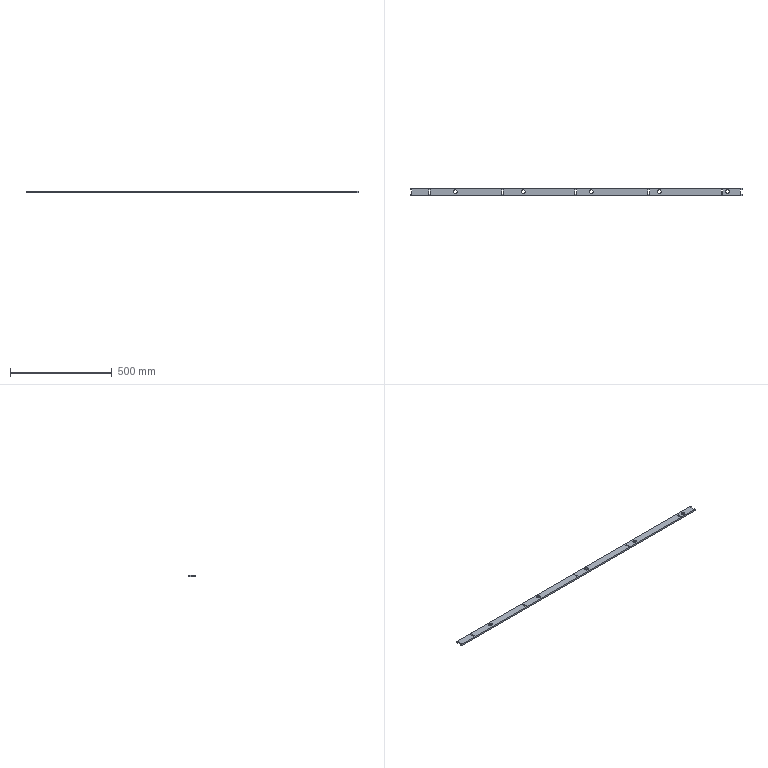Part | SolidWorks | features FlatPattern 1, SMBaseFlange 1, SheetMetal 1 | 1 solid | 44 faces | box 1635 x 34.8 x 8 mm | volume 435932 mm3 | plane 34 | cylinder 10 | commonest cylinder face diameters 18.1 x10
STEP:
#1=CARTESIAN_POINT('',(-81.05,53.917,8.));
#2=VERTEX_POINT('',#1);
#3=CARTESIAN_POINT('',(-62.95,53.917,8.));
#4=VERTEX_POINT('',#3);
#5=CARTESIAN_POINT('',(-72.,53.917,8.));
#6=DIRECTION('',(0.,0.,1.));
#7=DIRECTION('',(1.,0.,0.));
#8=AXIS2_PLACEMENT_3D('',#5,#6,#7);
#9=CIRCLE('',#8,9.05);
#10=EDGE_CURVE('',#2,#4,#9,.T.);
#11=ORIENTED_EDGE('',*,*,#10,.T.);
#12=CARTESIAN_POINT('',(-62.95,53.917,0.));
#13=VERTEX_POINT('',#12);
#14=CARTESIAN_POINT('',(-62.95,53.917,8.));
#15=DIRECTION('',(0.,0.,-1.));
#16=VECTOR('',#15,1000.);
#17=LINE('',#14,#16);
#18=EDGE_CURVE('',#4,#13,#17,.T.);
#19=ORIENTED_EDGE('',*,*,#18,.T.);
#20=CARTESIAN_POINT('',(-81.05,53.917,0.));
#21=VERTEX_POINT('',#20);
#22=CARTESIAN_POINT('',(-72.,53.917,0.));
#23=DIRECTION('',(0.,0.,1.));
#24=DIRECTION('',(1.,0.,0.));
#25=AXIS2_PLACEMENT_3D('',#22,#23,#24);
#26=CIRCLE('',#25,9.05);
#27=EDGE_CURVE('',#21,#13,#26,.T.);
#28=ORIENTED_EDGE('',*,*,#27,.F.);
#29=CARTESIAN_POINT('',(-81.05,53.917,8.));
#30=DIRECTION('',(0.,0.,-1.));
#31=VECTOR('',#30,1000.);
#32=LINE('',#29,#31);
#33=EDGE_CURVE('',#2,#21,#32,.T.);
#34=ORIENTED_EDGE('',*,*,#33,.F.);
#35=EDGE_LOOP('',(#11,#19,#28,#34));
#36=FACE_OUTER_BOUND('',#35,.T.);
#37=CARTESIAN_POINT('',(-72.,53.917,8.));
#38=DIRECTION('',(0.,0.,-1.));
#39=DIRECTION('',(-1.,0.,0.));
#40=AXIS2_PLACEMENT_3D('',#37,#38,#39);
#41=CYLINDRICAL_SURFACE('',#40,9.05);
#42=ADVANCED_FACE('',(#36),#41,.F.);
#43=CARTESIAN_POINT('',(-416.05,53.917,8.));
#44=VERTEX_POINT('',#43);
#45=CARTESIAN_POINT('',(-397.95,53.917,8.));
#46=VERTEX_POINT('',#45);
#47=CARTESIAN_POINT('',(-407.,53.917,8.));
#48=DIRECTION('',(0.,0.,1.));
#49=DIRECTION('',(1.,0.,0.));
#50=AXIS2_PLACEMENT_3D('',#47,#48,#49);
#51=CIRCLE('',#50,9.05);
#52=EDGE_CURVE('',#44,#46,#51,.T.);
#53=ORIENTED_EDGE('',*,*,#52,.T.);
#54=CARTESIAN_POINT('',(-397.95,53.917,0.));
#55=VERTEX_POINT('',#54);
#56=CARTESIAN_POINT('',(-397.95,53.917,8.));
#57=DIRECTION('',(0.,0.,-1.));
#58=VECTOR('',#57,1000.);
#59=LINE('',#56,#58);
#60=EDGE_CURVE('',#46,#55,#59,.T.);
#61=ORIENTED_EDGE('',*,*,#60,.T.);
#62=CARTESIAN_POINT('',(-416.05,53.917,0.));
#63=VERTEX_POINT('',#62);
#64=CARTESIAN_POINT('',(-407.,53.917,0.));
#65=DIRECTION('',(0.,0.,1.));
#66=DIRECTION('',(1.,0.,0.));
#67=AXIS2_PLACEMENT_3D('',#64,#65,#66);
#68=CIRCLE('',#67,9.05);
#69=EDGE_CURVE('',#63,#55,#68,.T.);
#70=ORIENTED_EDGE('',*,*,#69,.F.);
#71=CARTESIAN_POINT('',(-416.05,53.917,8.));
#72=DIRECTION('',(0.,0.,-1.));
#73=VECTOR('',#72,1000.);
#74=LINE('',#71,#73);
#75=EDGE_CURVE('',#44,#63,#74,.T.);
#76=ORIENTED_EDGE('',*,*,#75,.F.);
#77=EDGE_LOOP('',(#53,#61,#70,#76));
#78=FACE_OUTER_BOUND('',#77,.T.);
#79=CARTESIAN_POINT('',(-407.,53.917,8.));
#80=DIRECTION('',(0.,0.,-1.));
#81=DIRECTION('',(-1.,0.,0.));
#82=AXIS2_PLACEMENT_3D('',#79,#80,#81);
#83=CYLINDRICAL_SURFACE('',#82,9.05);
#84=ADVANCED_FACE('',(#78),#83,.F.);
#85=CARTESIAN_POINT('',(-751.05,53.917,8.));
#86=VERTEX_POINT('',#85);
#87=CARTESIAN_POINT('',(-732.95,53.917,8.));
#88=VERTEX_POINT('',#87);
#89=CARTESIAN_POINT('',(-742.,53.917,8.));
#90=DIRECTION('',(0.,0.,1.));
#91=DIRECTION('',(1.,0.,0.));
#92=AXIS2_PLACEMENT_3D('',#89,#90,#91);
#93=CIRCLE('',#92,9.05);
#94=EDGE_CURVE('',#86,#88,#93,.T.);
#95=ORIENTED_EDGE('',*,*,#94,.T.);
#96=CARTESIAN_POINT('',(-732.95,53.917,0.));
#97=VERTEX_POINT('',#96);
#98=CARTESIAN_POINT('',(-732.95,53.917,8.));
#99=DIRECTION('',(0.,0.,-1.));
#100=VECTOR('',#99,1000.);
#101=LINE('',#98,#100);
#102=EDGE_CURVE('',#88,#97,#101,.T.);
#103=ORIENTED_EDGE('',*,*,#102,.T.);
#104=CARTESIAN_POINT('',(-751.05,53.917,0.));
#105=VERTEX_POINT('',#104);
#106=CARTESIAN_POINT('',(-742.,53.917,0.));
#107=DIRECTION('',(0.,0.,1.));
#108=DIRECTION('',(1.,0.,0.));
#109=AXIS2_PLACEMENT_3D('',#106,#107,#108);
#110=CIRCLE('',#109,9.05);
#111=EDGE_CURVE('',#105,#97,#110,.T.);
#112=ORIENTED_EDGE('',*,*,#111,.F.);
#113=CARTESIAN_POINT('',(-751.05,53.917,8.));
#114=DIRECTION('',(0.,0.,-1.));
#115=VECTOR('',#114,1000.);
#116=LINE('',#113,#115);
#117=EDGE_CURVE('',#86,#105,#116,.T.);
#118=ORIENTED_EDGE('',*,*,#117,.F.);
#119=EDGE_LOOP('',(#95,#103,#112,#118));
#120=FACE_OUTER_BOUND('',#119,.T.);
#121=CARTESIAN_POINT('',(-742.,53.917,8.));
#122=DIRECTION('',(0.,0.,-1.));
#123=DIRECTION('',(-1.,0.,0.));
#124=AXIS2_PLACEMENT_3D('',#121,#122,#123);
#125=CYLINDRICAL_SURFACE('',#124,9.05);
#126=ADVANCED_FACE('',(#120),#125,.F.);
#127=CARTESIAN_POINT('',(-1086.05,53.917,8.));
#128=VERTEX_POINT('',#127);
#129=CARTESIAN_POINT('',(-1067.95,53.917,8.));
#130=VERTEX_POINT('',#129);
#131=CARTESIAN_POINT('',(-1077.,53.917,8.));
#132=DIRECTION('',(0.,0.,1.));
#133=DIRECTION('',(1.,0.,0.));
#134=AXIS2_PLACEMENT_3D('',#131,#132,#133);
#135=CIRCLE('',#134,9.05);
#136=EDGE_CURVE('',#128,#130,#135,.T.);
#137=ORIENTED_EDGE('',*,*,#136,.T.);
#138=CARTESIAN_POINT('',(-1067.95,53.917,0.));
#139=VERTEX_POINT('',#138);
#140=CARTESIAN_POINT('',(-1067.95,53.917,8.));
#141=DIRECTION('',(0.,0.,-1.));
#142=VECTOR('',#141,1000.);
#143=LINE('',#140,#142);
#144=EDGE_CURVE('',#130,#139,#143,.T.);
#145=ORIENTED_EDGE('',*,*,#144,.T.);
#146=CARTESIAN_POINT('',(-1086.05,53.917,0.));
#147=VERTEX_POINT('',#146);
#148=CARTESIAN_POINT('',(-1077.,53.917,0.));
#149=DIRECTION('',(0.,0.,1.));
#150=DIRECTION('',(1.,0.,0.));
#151=AXIS2_PLACEMENT_3D('',#148,#149,#150);
#152=CIRCLE('',#151,9.05);
#153=EDGE_CURVE('',#147,#139,#152,.T.);
#154=ORIENTED_EDGE('',*,*,#153,.F.);
#155=CARTESIAN_POINT('',(-1086.05,53.917,8.));
#156=DIRECTION('',(0.,0.,-1.));
#157=VECTOR('',#156,1000.);
#158=LINE('',#155,#157);
#159=EDGE_CURVE('',#128,#147,#158,.T.);
#160=ORIENTED_EDGE('',*,*,#159,.F.);
#161=EDGE_LOOP('',(#137,#145,#154,#160));
#162=FACE_OUTER_BOUND('',#161,.T.);
#163=CARTESIAN_POINT('',(-1077.,53.917,8.));
#164=DIRECTION('',(0.,0.,-1.));
#165=DIRECTION('',(-1.,0.,0.));
#166=AXIS2_PLACEMENT_3D('',#163,#164,#165);
#167=CYLINDRICAL_SURFACE('',#166,9.05);
#168=ADVANCED_FACE('',(#162),#167,.F.);
#169=CARTESIAN_POINT('',(-1421.05,53.917,8.));
#170=VERTEX_POINT('',#169);
#171=CARTESIAN_POINT('',(-1402.95,53.917,8.));
#172=VERTEX_POINT('',#171);
#173=CARTESIAN_POINT('',(-1412.,53.917,8.));
#174=DIRECTION('',(0.,0.,1.));
#175=DIRECTION('',(1.,0.,0.));
#176=AXIS2_PLACEMENT_3D('',#173,#174,#175);
#177=CIRCLE('',#176,9.05);
#178=EDGE_CURVE('',#170,#172,#177,.T.);
#179=ORIENTED_EDGE('',*,*,#178,.T.);
#180=CARTESIAN_POINT('',(-1402.95,53.917,0.));
#181=VERTEX_POINT('',#180);
#182=CARTESIAN_POINT('',(-1402.95,53.917,8.));
#183=DIRECTION('',(0.,0.,-1.));
#184=VECTOR('',#183,1000.);
#185=LINE('',#182,#184);
#186=EDGE_CURVE('',#172,#181,#185,.T.);
#187=ORIENTED_EDGE('',*,*,#186,.T.);
#188=CARTESIAN_POINT('',(-1421.05,53.917,0.));
#189=VERTEX_POINT('',#188);
#190=CARTESIAN_POINT('',(-1412.,53.917,0.));
#191=DIRECTION('',(0.,0.,1.));
#192=DIRECTION('',(1.,0.,0.));
#193=AXIS2_PLACEMENT_3D('',#190,#191,#192);
#194=CIRCLE('',#193,9.05);
#195=EDGE_CURVE('',#189,#181,#194,.T.);
#196=ORIENTED_EDGE('',*,*,#195,.F.);
#197=CARTESIAN_POINT('',(-1421.05,53.917,8.));
#198=DIRECTION('',(0.,0.,-1.));
#199=VECTOR('',#198,1000.);
#200=LINE('',#197,#199);
#201=EDGE_CURVE('',#170,#189,#200,.T.);
#202=ORIENTED_EDGE('',*,*,#201,.F.);
#203=EDGE_LOOP('',(#179,#187,#196,#202));
#204=FACE_OUTER_BOUND('',#203,.T.);
#205=CARTESIAN_POINT('',(-1412.,53.917,8.));
#206=DIRECTION('',(0.,0.,-1.));
#207=DIRECTION('',(-1.,0.,0.));
#208=AXIS2_PLACEMENT_3D('',#205,#206,#207);
#209=CYLINDRICAL_SURFACE('',#208,9.05);
#210=ADVANCED_FACE('',(#204),#209,.F.);
#211=ORIENTED_EDGE('',*,*,#52,.F.);
#212=CARTESIAN_POINT('',(-407.,53.917,8.));
#213=DIRECTION('',(0.,0.,1.));
#214=DIRECTION('',(1.,0.,0.));
#215=AXIS2_PLACEMENT_3D('',#212,#213,#214);
#216=CIRCLE('',#215,9.05);
#217=EDGE_CURVE('',#46,#44,#216,.T.);
#218=ORIENTED_EDGE('',*,*,#217,.F.);
#219=EDGE_LOOP('',(#211,#218));
#220=FACE_BOUND('',#219,.T.);
#221=ORIENTED_EDGE('',*,*,#136,.F.);
#222=CARTESIAN_POINT('',(-1077.,53.917,8.));
#223=DIRECTION('',(0.,0.,1.));
#224=DIRECTION('',(1.,0.,0.));
#225=AXIS2_PLACEMENT_3D('',#222,#223,#224);
#226=CIRCLE('',#225,9.05);
#227=EDGE_CURVE('',#130,#128,#226,.T.);
#228=ORIENTED_EDGE('',*,*,#227,.F.);
#229=EDGE_LOOP('',(#221,#228));
#230=FACE_BOUND('',#229,.T.);
#231=CARTESIAN_POINT('',(0.,62.417,8.));
#232=VERTEX_POINT('',#231);
#233=CARTESIAN_POINT('',(0.,69.917,8.));
#234=VERTEX_POINT('',#233);
#235=CARTESIAN_POINT('',(0.,69.917,8.));
#236=DIRECTION('',(0.,1.,0.));
#237=VECTOR('',#236,1000.);
#238=LINE('',#235,#237);
#239=EDGE_CURVE('',#232,#234,#238,.T.);
#240=ORIENTED_EDGE('',*,*,#239,.T.);
#241=CARTESIAN_POINT('',(-1635.,69.917,8.));
#242=VERTEX_POINT('',#241);
#243=CARTESIAN_POINT('',(0.,69.917,8.));
#244=DIRECTION('',(-1.,0.,0.));
#245=VECTOR('',#244,1000.);
#246=LINE('',#243,#245);
#247=EDGE_CURVE('',#234,#242,#246,.T.);
#248=ORIENTED_EDGE('',*,*,#247,.T.);
#249=CARTESIAN_POINT('',(-1635.,62.417,8.));
#250=VERTEX_POINT('',#249);
#251=CARTESIAN_POINT('',(-1635.,69.917,8.));
#252=DIRECTION('',(0.,-1.,0.));
#253=VECTOR('',#252,1000.);
#254=LINE('',#251,#253);
#255=EDGE_CURVE('',#242,#250,#254,.T.);
#256=ORIENTED_EDGE('',*,*,#255,.T.);
#257=CARTESIAN_POINT('',(-1627.,62.417,8.));
#258=VERTEX_POINT('',#257);
#259=CARTESIAN_POINT('',(-1627.,62.417,8.));
#260=DIRECTION('',(1.,0.,0.));
#261=VECTOR('',#260,1000.);
#262=LINE('',#259,#261);
#263=EDGE_CURVE('',#250,#258,#262,.T.);
#264=ORIENTED_EDGE('',*,*,#263,.T.);
#265=CARTESIAN_POINT('',(-1627.,42.417,8.));
#266=VERTEX_POINT('',#265);
#267=CARTESIAN_POINT('',(-1627.,62.417,8.));
#268=DIRECTION('',(0.,-1.,0.));
#269=VECTOR('',#268,1000.);
#270=LINE('',#267,#269);
#271=EDGE_CURVE('',#258,#266,#270,.T.);
#272=ORIENTED_EDGE('',*,*,#271,.T.);
#273=CARTESIAN_POINT('',(-1635.,42.417,8.));
#274=VERTEX_POINT('',#273);
#275=CARTESIAN_POINT('',(-1627.,42.417,8.));
#276=DIRECTION('',(-1.,0.,0.));
#277=VECTOR('',#276,1000.);
#278=LINE('',#275,#277);
#279=EDGE_CURVE('',#266,#274,#278,.T.);
#280=ORIENTED_EDGE('',*,*,#279,.T.);
#281=CARTESIAN_POINT('',(-1635.,35.117,8.));
#282=VERTEX_POINT('',#281);
#283=CARTESIAN_POINT('',(-1635.,42.417,8.));
#284=DIRECTION('',(0.,-1.,0.));
#285=VECTOR('',#284,1000.);
#286=LINE('',#283,#285);
#287=EDGE_CURVE('',#274,#282,#286,.T.);
#288=ORIENTED_EDGE('',*,*,#287,.T.);
#289=CARTESIAN_POINT('',(0.,35.117,8.));
#290=VERTEX_POINT('',#289);
#291=CARTESIAN_POINT('',(0.,35.117,8.));
#292=DIRECTION('',(1.,0.,0.));
#293=VECTOR('',#292,1000.);
#294=LINE('',#291,#293);
#295=EDGE_CURVE('',#282,#290,#294,.T.);
#296=ORIENTED_EDGE('',*,*,#295,.T.);
#297=CARTESIAN_POINT('',(0.,42.417,8.));
#298=VERTEX_POINT('',#297);
#299=CARTESIAN_POINT('',(0.,42.417,8.));
#300=DIRECTION('',(0.,1.,0.));
#301=VECTOR('',#300,1000.);
#302=LINE('',#299,#301);
#303=EDGE_CURVE('',#290,#298,#302,.T.);
#304=ORIENTED_EDGE('',*,*,#303,.T.);
#305=CARTESIAN_POINT('',(-8.,42.417,8.));
#306=VERTEX_POINT('',#305);
#307=CARTESIAN_POINT('',(-8.,42.417,8.));
#308=DIRECTION('',(-1.,0.,0.));
#309=VECTOR('',#308,1000.);
#310=LINE('',#307,#309);
#311=EDGE_CURVE('',#298,#306,#310,.T.);
#312=ORIENTED_EDGE('',*,*,#311,.T.);
#313=CARTESIAN_POINT('',(-8.,62.417,8.));
#314=VERTEX_POINT('',#313);
#315=CARTESIAN_POINT('',(-8.,62.417,8.));
#316=DIRECTION('',(0.,1.,0.));
#317=VECTOR('',#316,1000.);
#318=LINE('',#315,#317);
#319=EDGE_CURVE('',#306,#314,#318,.T.);
#320=ORIENTED_EDGE('',*,*,#319,.T.);
#321=CARTESIAN_POINT('',(-8.,62.417,8.));
#322=DIRECTION('',(1.,0.,0.));
#323=VECTOR('',#322,1000.);
#324=LINE('',#321,#323);
#325=EDGE_CURVE('',#314,#232,#324,.T.);
#326=ORIENTED_EDGE('',*,*,#325,.T.);
#327=EDGE_LOOP('',(#240,#248,#256,#264,#272,#280,#288,#296,#304,#312,#320,#326));
#328=FACE_OUTER_BOUND('',#327,.T.);
#329=ORIENTED_EDGE('',*,*,#178,.F.);
#330=CARTESIAN_POINT('',(-1412.,53.917,8.));
#331=DIRECTION('',(0.,0.,1.));
#332=DIRECTION('',(1.,0.,0.));
#333=AXIS2_PLACEMENT_3D('',#330,#331,#332);
#334=CIRCLE('',#333,9.05);
#335=EDGE_CURVE('',#172,#170,#334,.T.);
#336=ORIENTED_EDGE('',*,*,#335,.F.);
#337=EDGE_LOOP('',(#329,#336));
#338=FACE_BOUND('',#337,.T.);
#339=ORIENTED_EDGE('',*,*,#94,.F.);
#340=CARTESIAN_POINT('',(-742.,53.917,8.));
#341=DIRECTION('',(0.,0.,1.));
#342=DIRECTION('',(1.,0.,0.));
#343=AXIS2_PLACEMENT_3D('',#340,#341,#342);
#344=CIRCLE('',#343,9.05);
#345=EDGE_CURVE('',#88,#86,#344,.T.);
#346=ORIENTED_EDGE('',*,*,#345,.F.);
#347=EDGE_LOOP('',(#339,#346));
#348=FACE_BOUND('',#347,.T.);
#349=ORIENTED_EDGE('',*,*,#10,.F.);
#350=CARTESIAN_POINT('',(-72.,53.917,8.));
#351=DIRECTION('',(0.,0.,1.));
#352=DIRECTION('',(1.,0.,0.));
#353=AXIS2_PLACEMENT_3D('',#350,#351,#352);
#354=CIRCLE('',#353,9.05);
#355=EDGE_CURVE('',#4,#2,#354,.T.);
#356=ORIENTED_EDGE('',*,*,#355,.F.);
#357=EDGE_LOOP('',(#349,#356));
#358=FACE_BOUND('',#357,.T.);
#359=CARTESIAN_POINT('',(-95.,62.417,8.));
#360=VERTEX_POINT('',#359);
#361=CARTESIAN_POINT('',(-103.,62.417,8.));
#362=VERTEX_POINT('',#361);
#363=CARTESIAN_POINT('',(-95.,62.417,8.));
#364=DIRECTION('',(-1.,0.,0.));
#365=VECTOR('',#364,1000.);
#366=LINE('',#363,#365);
#367=EDGE_CURVE('',#360,#362,#366,.T.);
#368=ORIENTED_EDGE('',*,*,#367,.F.);
#369=CARTESIAN_POINT('',(-95.,42.417,8.));
#370=VERTEX_POINT('',#369);
#371=CARTESIAN_POINT('',(-95.,62.417,8.));
#372=DIRECTION('',(0.,1.,0.));
#373=VECTOR('',#372,1000.);
#374=LINE('',#371,#373);
#375=EDGE_CURVE('',#370,#360,#374,.T.);
#376=ORIENTED_EDGE('',*,*,#375,.F.);
#377=CARTESIAN_POINT('',(-103.,42.417,8.));
#378=VERTEX_POINT('',#377);
#379=CARTESIAN_POINT('',(-95.,42.417,8.));
#380=DIRECTION('',(1.,0.,0.));
#381=VECTOR('',#380,1000.);
#382=LINE('',#379,#381);
#383=EDGE_CURVE('',#378,#370,#382,.T.);
#384=ORIENTED_EDGE('',*,*,#383,.F.);
#385=CARTESIAN_POINT('',(-103.,62.417,8.));
#386=DIRECTION('',(0.,-1.,0.));
#387=VECTOR('',#386,1000.);
#388=LINE('',#385,#387);
#389=EDGE_CURVE('',#362,#378,#388,.T.);
#390=ORIENTED_EDGE('',*,*,#389,.F.);
#391=EDGE_LOOP('',(#368,#376,#384,#390));
#392=FACE_BOUND('',#391,.T.);
#393=CARTESIAN_POINT('',(-455.,62.417,8.));
#394=VERTEX_POINT('',#393);
#395=CARTESIAN_POINT('',(-463.,62.417,8.));
#396=VERTEX_POINT('',#395);
#397=CARTESIAN_POINT('',(-455.,62.417,8.));
#398=DIRECTION('',(-1.,0.,0.));
#399=VECTOR('',#398,1000.);
#400=LINE('',#397,#399);
#401=EDGE_CURVE('',#394,#396,#400,.T.);
#402=ORIENTED_EDGE('',*,*,#401,.F.);
#403=CARTESIAN_POINT('',(-455.,42.417,8.));
#404=VERTEX_POINT('',#403);
#405=CARTESIAN_POINT('',(-455.,62.417,8.));
#406=DIRECTION('',(0.,1.,0.));
#407=VECTOR('',#406,1000.);
#408=LINE('',#405,#407);
#409=EDGE_CURVE('',#404,#394,#408,.T.);
#410=ORIENTED_EDGE('',*,*,#409,.F.);
#411=CARTESIAN_POINT('',(-463.,42.417,8.));
#412=VERTEX_POINT('',#411);
#413=CARTESIAN_POINT('',(-455.,42.417,8.));
#414=DIRECTION('',(1.,0.,0.));
#415=VECTOR('',#414,1000.);
#416=LINE('',#413,#415);
#417=EDGE_CURVE('',#412,#404,#416,.T.);
#418=ORIENTED_EDGE('',*,*,#417,.F.);
#419=CARTESIAN_POINT('',(-463.,62.417,8.));
#420=DIRECTION('',(0.,-1.,0.));
#421=VECTOR('',#420,1000.);
#422=LINE('',#419,#421);
#423=EDGE_CURVE('',#396,#412,#422,.T.);
#424=ORIENTED_EDGE('',*,*,#423,.F.);
#425=EDGE_LOOP('',(#402,#410,#418,#424));
#426=FACE_BOUND('',#425,.T.);
#427=CARTESIAN_POINT('',(-815.,62.417,8.));
#428=VERTEX_POINT('',#427);
#429=CARTESIAN_POINT('',(-823.,62.417,8.));
#430=VERTEX_POINT('',#429);
#431=CARTESIAN_POINT('',(-815.,62.417,8.));
#432=DIRECTION('',(-1.,0.,0.));
#433=VECTOR('',#432,1000.);
#434=LINE('',#431,#433);
#435=EDGE_CURVE('',#428,#430,#434,.T.);
#436=ORIENTED_EDGE('',*,*,#435,.F.);
#437=CARTESIAN_POINT('',(-815.,42.417,8.));
#438=VERTEX_POINT('',#437);
#439=CARTESIAN_POINT('',(-815.,62.417,8.));
#440=DIRECTION('',(0.,1.,0.));
#441=VECTOR('',#440,1000.);
#442=LINE('',#439,#441);
#443=EDGE_CURVE('',#438,#428,#442,.T.);
#444=ORIENTED_EDGE('',*,*,#443,.F.);
#445=CARTESIAN_POINT('',(-823.,42.417,8.));
#446=VERTEX_POINT('',#445);
#447=CARTESIAN_POINT('',(-815.,42.417,8.));
#448=DIRECTION('',(1.,0.,0.));
#449=VECTOR('',#448,1000.);
#450=LINE('',#447,#449);
#451=EDGE_CURVE('',#446,#438,#450,.T.);
#452=ORIENTED_EDGE('',*,*,#451,.F.);
#453=CARTESIAN_POINT('',(-823.,62.417,8.));
#454=DIRECTION('',(0.,-1.,0.));
#455=VECTOR('',#454,1000.);
#456=LINE('',#453,#455);
#457=EDGE_CURVE('',#430,#446,#456,.T.);
#458=ORIENTED_EDGE('',*,*,#457,.F.);
#459=EDGE_LOOP('',(#436,#444,#452,#458));
#460=FACE_BOUND('',#459,.T.);
#461=CARTESIAN_POINT('',(-1175.,62.417,8.));
#462=VERTEX_POINT('',#461);
#463=CARTESIAN_POINT('',(-1183.,62.417,8.));
#464=VERTEX_POINT('',#463);
#465=CARTESIAN_POINT('',(-1175.,62.417,8.));
#466=DIRECTION('',(-1.,0.,0.));
#467=VECTOR('',#466,1000.);
#468=LINE('',#465,#467);
#469=EDGE_CURVE('',#462,#464,#468,.T.);
#470=ORIENTED_EDGE('',*,*,#469,.F.);
#471=CARTESIAN_POINT('',(-1175.,42.417,8.));
#472=VERTEX_POINT('',#471);
#473=CARTESIAN_POINT('',(-1175.,62.417,8.));
#474=DIRECTION('',(0.,1.,0.));
#475=VECTOR('',#474,1000.);
#476=LINE('',#473,#475);
#477=EDGE_CURVE('',#472,#462,#476,.T.);
#478=ORIENTED_EDGE('',*,*,#477,.F.);
#479=CARTESIAN_POINT('',(-1183.,42.417,8.));
#480=VERTEX_POINT('',#479);
#481=CARTESIAN_POINT('',(-1175.,42.417,8.));
#482=DIRECTION('',(1.,0.,0.));
#483=VECTOR('',#482,1000.);
#484=LINE('',#481,#483);
#485=EDGE_CURVE('',#480,#472,#484,.T.);
#486=ORIENTED_EDGE('',*,*,#485,.F.);
#487=CARTESIAN_POINT('',(-1183.,62.417,8.));
#488=DIRECTION('',(0.,-1.,0.));
#489=VECTOR('',#488,1000.);
#490=LINE('',#487,#489);
#491=EDGE_CURVE('',#464,#480,#490,.T.);
#492=ORIENTED_EDGE('',*,*,#491,.F.);
#493=EDGE_LOOP('',(#470,#478,#486,#492));
#494=FACE_BOUND('',#493,.T.);
#495=CARTESIAN_POINT('',(-1535.,62.417,8.));
#496=VERTEX_POINT('',#495);
#497=CARTESIAN_POINT('',(-1543.,62.417,8.));
#498=VERTEX_POINT('',#497);
#499=CARTESIAN_POINT('',(-1535.,62.417,8.));
#500=DIRECTION('',(-1.,0.,0.));
#501=VECTOR('',#500,1000.);
#502=LINE('',#499,#501);
#503=EDGE_CURVE('',#496,#498,#502,.T.);
#504=ORIENTED_EDGE('',*,*,#503,.F.);
#505=CARTESIAN_POINT('',(-1535.,42.417,8.));
#506=VERTEX_POINT('',#505);
#507=CARTESIAN_POINT('',(-1535.,62.417,8.));
#508=DIRECTION('',(0.,1.,0.));
#509=VECTOR('',#508,1000.);
#510=LINE('',#507,#509);
#511=EDGE_CURVE('',#506,#496,#510,.T.);
#512=ORIENTED_EDGE('',*,*,#511,.F.);
#513=CARTESIAN_POINT('',(-1543.,42.417,8.));
#514=VERTEX_POINT('',#513);
#515=CARTESIAN_POINT('',(-1535.,42.417,8.));
#516=DIRECTION('',(1.,0.,0.));
#517=VECTOR('',#516,1000.);
#518=LINE('',#515,#517);
#519=EDGE_CURVE('',#514,#506,#518,.T.);
#520=ORIENTED_EDGE('',*,*,#519,.F.);
#521=CARTESIAN_POINT('',(-1543.,62.417,8.));
#522=DIRECTION('',(0.,-1.,0.));
#523=VECTOR('',#522,1000.);
#524=LINE('',#521,#523);
#525=EDGE_CURVE('',#498,#514,#524,.T.);
#526=ORIENTED_EDGE('',*,*,#525,.F.);
#527=EDGE_LOOP('',(#504,#512,#520,#526));
#528=FACE_BOUND('',#527,.T.);
#529=CARTESIAN_POINT('',(0.,0.,8.));
#530=DIRECTION('',(0.,0.,1.));
#531=DIRECTION('',(1.,0.,0.));
#532=AXIS2_PLACEMENT_3D('',#529,#530,#531);
#533=PLANE('',#532);
#534=ADVANCED_FACE('',(#220,#230,#328,#338,#348,#358,#392,#426,#460,#494,#528),#533,.T.);
#535=CARTESIAN_POINT('',(-1175.,42.417,0.));
#536=VERTEX_POINT('',#535);
#537=CARTESIAN_POINT('',(-1175.,62.417,0.));
#538=VERTEX_POINT('',#537);
#539=CARTESIAN_POINT('',(-1175.,62.417,0.));
#540=DIRECTION('',(0.,1.,0.));
#541=VECTOR('',#540,1000.);
#542=LINE('',#539,#541);
#543=EDGE_CURVE('',#536,#538,#542,.T.);
#544=ORIENTED_EDGE('',*,*,#543,.T.);
#545=CARTESIAN_POINT('',(-1183.,62.417,0.));
#546=VERTEX_POINT('',#545);
#547=CARTESIAN_POINT('',(-1175.,62.417,0.));
#548=DIRECTION('',(-1.,0.,0.));
#549=VECTOR('',#548,1000.);
#550=LINE('',#547,#549);
#551=EDGE_CURVE('',#538,#546,#550,.T.);
#552=ORIENTED_EDGE('',*,*,#551,.T.);
#553=CARTESIAN_POINT('',(-1183.,42.417,0.));
#554=VERTEX_POINT('',#553);
#555=CARTESIAN_POINT('',(-1183.,62.417,0.));
#556=DIRECTION('',(0.,-1.,0.));
#557=VECTOR('',#556,1000.);
#558=LINE('',#555,#557);
#559=EDGE_CURVE('',#546,#554,#558,.T.);
#560=ORIENTED_EDGE('',*,*,#559,.T.);
#561=CARTESIAN_POINT('',(-1175.,42.417,0.));
#562=DIRECTION('',(1.,0.,0.));
#563=VECTOR('',#562,1000.);
#564=LINE('',#561,#563);
#565=EDGE_CURVE('',#554,#536,#564,.T.);
#566=ORIENTED_EDGE('',*,*,#565,.T.);
#567=EDGE_LOOP('',(#544,#552,#560,#566));
#568=FACE_BOUND('',#567,.T.);
#569=CARTESIAN_POINT('',(-455.,42.417,0.));
#570=VERTEX_POINT('',#569);
#571=CARTESIAN_POINT('',(-455.,62.417,0.));
#572=VERTEX_POINT('',#571);
#573=CARTESIAN_POINT('',(-455.,62.417,0.));
#574=DIRECTION('',(0.,1.,0.));
#575=VECTOR('',#574,1000.);
#576=LINE('',#573,#575);
#577=EDGE_CURVE('',#570,#572,#576,.T.);
#578=ORIENTED_EDGE('',*,*,#577,.T.);
#579=CARTESIAN_POINT('',(-463.,62.417,0.));
#580=VERTEX_POINT('',#579);
#581=CARTESIAN_POINT('',(-455.,62.417,0.));
#582=DIRECTION('',(-1.,0.,0.));
#583=VECTOR('',#582,1000.);
#584=LINE('',#581,#583);
#585=EDGE_CURVE('',#572,#580,#584,.T.);
#586=ORIENTED_EDGE('',*,*,#585,.T.);
#587=CARTESIAN_POINT('',(-463.,42.417,0.));
#588=VERTEX_POINT('',#587);
#589=CARTESIAN_POINT('',(-463.,62.417,0.));
#590=DIRECTION('',(0.,-1.,0.));
#591=VECTOR('',#590,1000.);
#592=LINE('',#589,#591);
#593=EDGE_CURVE('',#580,#588,#592,.T.);
#594=ORIENTED_EDGE('',*,*,#593,.T.);
#595=CARTESIAN_POINT('',(-455.,42.417,0.));
#596=DIRECTION('',(1.,0.,0.));
#597=VECTOR('',#596,1000.);
#598=LINE('',#595,#597);
#599=EDGE_CURVE('',#588,#570,#598,.T.);
#600=ORIENTED_EDGE('',*,*,#599,.T.);
#601=EDGE_LOOP('',(#578,#586,#594,#600));
#602=FACE_BOUND('',#601,.T.);
#603=ORIENTED_EDGE('',*,*,#27,.T.);
#604=CARTESIAN_POINT('',(-72.,53.917,0.));
#605=DIRECTION('',(0.,0.,1.));
#606=DIRECTION('',(1.,0.,0.));
#607=AXIS2_PLACEMENT_3D('',#604,#605,#606);
#608=CIRCLE('',#607,9.05);
#609=EDGE_CURVE('',#13,#21,#608,.T.);
#610=ORIENTED_EDGE('',*,*,#609,.T.);
#611=EDGE_LOOP('',(#603,#610));
#612=FACE_BOUND('',#611,.T.);
#613=ORIENTED_EDGE('',*,*,#69,.T.);
#614=CARTESIAN_POINT('',(-407.,53.917,0.));
#615=DIRECTION('',(0.,0.,1.));
#616=DIRECTION('',(1.,0.,0.));
#617=AXIS2_PLACEMENT_3D('',#614,#615,#616);
#618=CIRCLE('',#617,9.05);
#619=EDGE_CURVE('',#55,#63,#618,.T.);
#620=ORIENTED_EDGE('',*,*,#619,.T.);
#621=EDGE_LOOP('',(#613,#620));
#622=FACE_BOUND('',#621,.T.);
#623=ORIENTED_EDGE('',*,*,#111,.T.);
#624=CARTESIAN_POINT('',(-742.,53.917,0.));
#625=DIRECTION('',(0.,0.,1.));
#626=DIRECTION('',(1.,0.,0.));
#627=AXIS2_PLACEMENT_3D('',#624,#625,#626);
#628=CIRCLE('',#627,9.05);
#629=EDGE_CURVE('',#97,#105,#628,.T.);
#630=ORIENTED_EDGE('',*,*,#629,.T.);
#631=EDGE_LOOP('',(#623,#630));
#632=FACE_BOUND('',#631,.T.);
#633=ORIENTED_EDGE('',*,*,#153,.T.);
#634=CARTESIAN_POINT('',(-1077.,53.917,0.));
#635=DIRECTION('',(0.,0.,1.));
#636=DIRECTION('',(1.,0.,0.));
#637=AXIS2_PLACEMENT_3D('',#634,#635,#636);
#638=CIRCLE('',#637,9.05);
#639=EDGE_CURVE('',#139,#147,#638,.T.);
#640=ORIENTED_EDGE('',*,*,#639,.T.);
#641=EDGE_LOOP('',(#633,#640));
#642=FACE_BOUND('',#641,.T.);
#643=ORIENTED_EDGE('',*,*,#195,.T.);
#644=CARTESIAN_POINT('',(-1412.,53.917,0.));
#645=DIRECTION('',(0.,0.,1.));
#646=DIRECTION('',(1.,0.,0.));
#647=AXIS2_PLACEMENT_3D('',#644,#645,#646);
#648=CIRCLE('',#647,9.05);
#649=EDGE_CURVE('',#181,#189,#648,.T.);
#650=ORIENTED_EDGE('',*,*,#649,.T.);
#651=EDGE_LOOP('',(#643,#650));
#652=FACE_BOUND('',#651,.T.);
#653=CARTESIAN_POINT('',(0.,62.417,0.));
#654=VERTEX_POINT('',#653);
#655=CARTESIAN_POINT('',(0.,69.917,0.));
#656=VERTEX_POINT('',#655);
#657=CARTESIAN_POINT('',(0.,69.917,0.));
#658=DIRECTION('',(0.,1.,0.));
#659=VECTOR('',#658,1000.);
#660=LINE('',#657,#659);
#661=EDGE_CURVE('',#654,#656,#660,.T.);
#662=ORIENTED_EDGE('',*,*,#661,.F.);
#663=CARTESIAN_POINT('',(-8.,62.417,0.));
#664=VERTEX_POINT('',#663);
#665=CARTESIAN_POINT('',(-8.,62.417,0.));
#666=DIRECTION('',(1.,0.,0.));
#667=VECTOR('',#666,1000.);
#668=LINE('',#665,#667);
#669=EDGE_CURVE('',#664,#654,#668,.T.);
#670=ORIENTED_EDGE('',*,*,#669,.F.);
#671=CARTESIAN_POINT('',(-8.,42.417,0.));
#672=VERTEX_POINT('',#671);
#673=CARTESIAN_POINT('',(-8.,62.417,0.));
#674=DIRECTION('',(0.,1.,0.));
#675=VECTOR('',#674,1000.);
#676=LINE('',#673,#675);
#677=EDGE_CURVE('',#672,#664,#676,.T.);
#678=ORIENTED_EDGE('',*,*,#677,.F.);
#679=CARTESIAN_POINT('',(0.,42.417,0.));
#680=VERTEX_POINT('',#679);
#681=CARTESIAN_POINT('',(-8.,42.417,0.));
#682=DIRECTION('',(-1.,0.,0.));
#683=VECTOR('',#682,1000.);
#684=LINE('',#681,#683);
#685=EDGE_CURVE('',#680,#672,#684,.T.);
#686=ORIENTED_EDGE('',*,*,#685,.F.);
#687=CARTESIAN_POINT('',(0.,35.117,0.));
#688=VERTEX_POINT('',#687);
#689=CARTESIAN_POINT('',(0.,42.417,0.));
#690=DIRECTION('',(0.,1.,0.));
#691=VECTOR('',#690,1000.);
#692=LINE('',#689,#691);
#693=EDGE_CURVE('',#688,#680,#692,.T.);
#694=ORIENTED_EDGE('',*,*,#693,.F.);
#695=CARTESIAN_POINT('',(-1635.,35.117,0.));
#696=VERTEX_POINT('',#695);
#697=CARTESIAN_POINT('',(0.,35.117,0.));
#698=DIRECTION('',(1.,0.,0.));
#699=VECTOR('',#698,1000.);
#700=LINE('',#697,#699);
#701=EDGE_CURVE('',#696,#688,#700,.T.);
#702=ORIENTED_EDGE('',*,*,#701,.F.);
#703=CARTESIAN_POINT('',(-1635.,42.417,0.));
#704=VERTEX_POINT('',#703);
#705=CARTESIAN_POINT('',(-1635.,42.417,0.));
#706=DIRECTION('',(0.,-1.,0.));
#707=VECTOR('',#706,1000.);
#708=LINE('',#705,#707);
#709=EDGE_CURVE('',#704,#696,#708,.T.);
#710=ORIENTED_EDGE('',*,*,#709,.F.);
#711=CARTESIAN_POINT('',(-1627.,42.417,0.));
#712=VERTEX_POINT('',#711);
#713=CARTESIAN_POINT('',(-1627.,42.417,0.));
#714=DIRECTION('',(-1.,0.,0.));
#715=VECTOR('',#714,1000.);
#716=LINE('',#713,#715);
#717=EDGE_CURVE('',#712,#704,#716,.T.);
#718=ORIENTED_EDGE('',*,*,#717,.F.);
#719=CARTESIAN_POINT('',(-1627.,62.417,0.));
#720=VERTEX_POINT('',#719);
#721=CARTESIAN_POINT('',(-1627.,62.417,0.));
#722=DIRECTION('',(0.,-1.,0.));
#723=VECTOR('',#722,1000.);
#724=LINE('',#721,#723);
#725=EDGE_CURVE('',#720,#712,#724,.T.);
#726=ORIENTED_EDGE('',*,*,#725,.F.);
#727=CARTESIAN_POINT('',(-1635.,62.417,0.));
#728=VERTEX_POINT('',#727);
#729=CARTESIAN_POINT('',(-1627.,62.417,0.));
#730=DIRECTION('',(1.,0.,0.));
#731=VECTOR('',#730,1000.);
#732=LINE('',#729,#731);
#733=EDGE_CURVE('',#728,#720,#732,.T.);
#734=ORIENTED_EDGE('',*,*,#733,.F.);
#735=CARTESIAN_POINT('',(-1635.,69.917,0.));
#736=VERTEX_POINT('',#735);
#737=CARTESIAN_POINT('',(-1635.,69.917,0.));
#738=DIRECTION('',(0.,-1.,0.));
#739=VECTOR('',#738,1000.);
#740=LINE('',#737,#739);
#741=EDGE_CURVE('',#736,#728,#740,.T.);
#742=ORIENTED_EDGE('',*,*,#741,.F.);
#743=CARTESIAN_POINT('',(0.,69.917,0.));
#744=DIRECTION('',(-1.,0.,0.));
#745=VECTOR('',#744,1000.);
#746=LINE('',#743,#745);
#747=EDGE_CURVE('',#656,#736,#746,.T.);
#748=ORIENTED_EDGE('',*,*,#747,.F.);
#749=EDGE_LOOP('',(#662,#670,#678,#686,#694,#702,#710,#718,#726,#734,#742,#748));
#750=FACE_OUTER_BOUND('',#749,.T.);
#751=CARTESIAN_POINT('',(-95.,42.417,0.));
#752=VERTEX_POINT('',#751);
#753=CARTESIAN_POINT('',(-95.,62.417,0.));
#754=VERTEX_POINT('',#753);
#755=CARTESIAN_POINT('',(-95.,62.417,0.));
#756=DIRECTION('',(0.,1.,0.));
#757=VECTOR('',#756,1000.);
#758=LINE('',#755,#757);
#759=EDGE_CURVE('',#752,#754,#758,.T.);
#760=ORIENTED_EDGE('',*,*,#759,.T.);
#761=CARTESIAN_POINT('',(-103.,62.417,0.));
#762=VERTEX_POINT('',#761);
#763=CARTESIAN_POINT('',(-95.,62.417,0.));
#764=DIRECTION('',(-1.,0.,0.));
#765=VECTOR('',#764,1000.);
#766=LINE('',#763,#765);
#767=EDGE_CURVE('',#754,#762,#766,.T.);
#768=ORIENTED_EDGE('',*,*,#767,.T.);
#769=CARTESIAN_POINT('',(-103.,42.417,0.));
#770=VERTEX_POINT('',#769);
#771=CARTESIAN_POINT('',(-103.,62.417,0.));
#772=DIRECTION('',(0.,-1.,0.));
#773=VECTOR('',#772,1000.);
#774=LINE('',#771,#773);
#775=EDGE_CURVE('',#762,#770,#774,.T.);
#776=ORIENTED_EDGE('',*,*,#775,.T.);
#777=CARTESIAN_POINT('',(-95.,42.417,0.));
#778=DIRECTION('',(1.,0.,0.));
#779=VECTOR('',#778,1000.);
#780=LINE('',#777,#779);
#781=EDGE_CURVE('',#770,#752,#780,.T.);
#782=ORIENTED_EDGE('',*,*,#781,.T.);
#783=EDGE_LOOP('',(#760,#768,#776,#782));
#784=FACE_BOUND('',#783,.T.);
#785=CARTESIAN_POINT('',(-815.,42.417,0.));
#786=VERTEX_POINT('',#785);
#787=CARTESIAN_POINT('',(-815.,62.417,0.));
#788=VERTEX_POINT('',#787);
#789=CARTESIAN_POINT('',(-815.,62.417,0.));
#790=DIRECTION('',(0.,1.,0.));
#791=VECTOR('',#790,1000.);
#792=LINE('',#789,#791);
#793=EDGE_CURVE('',#786,#788,#792,.T.);
#794=ORIENTED_EDGE('',*,*,#793,.T.);
#795=CARTESIAN_POINT('',(-823.,62.417,0.));
#796=VERTEX_POINT('',#795);
#797=CARTESIAN_POINT('',(-815.,62.417,0.));
#798=DIRECTION('',(-1.,0.,0.));
#799=VECTOR('',#798,1000.);
#800=LINE('',#797,#799);
#801=EDGE_CURVE('',#788,#796,#800,.T.);
#802=ORIENTED_EDGE('',*,*,#801,.T.);
#803=CARTESIAN_POINT('',(-823.,42.417,0.));
#804=VERTEX_POINT('',#803);
#805=CARTESIAN_POINT('',(-823.,62.417,0.));
#806=DIRECTION('',(0.,-1.,0.));
#807=VECTOR('',#806,1000.);
#808=LINE('',#805,#807);
#809=EDGE_CURVE('',#796,#804,#808,.T.);
#810=ORIENTED_EDGE('',*,*,#809,.T.);
#811=CARTESIAN_POINT('',(-815.,42.417,0.));
#812=DIRECTION('',(1.,0.,0.));
#813=VECTOR('',#812,1000.);
#814=LINE('',#811,#813);
#815=EDGE_CURVE('',#804,#786,#814,.T.);
#816=ORIENTED_EDGE('',*,*,#815,.T.);
#817=EDGE_LOOP('',(#794,#802,#810,#816));
#818=FACE_BOUND('',#817,.T.);
#819=CARTESIAN_POINT('',(-1535.,42.417,0.));
#820=VERTEX_POINT('',#819);
#821=CARTESIAN_POINT('',(-1535.,62.417,0.));
#822=VERTEX_POINT('',#821);
#823=CARTESIAN_POINT('',(-1535.,62.417,0.));
#824=DIRECTION('',(0.,1.,0.));
#825=VECTOR('',#824,1000.);
#826=LINE('',#823,#825);
#827=EDGE_CURVE('',#820,#822,#826,.T.);
#828=ORIENTED_EDGE('',*,*,#827,.T.);
#829=CARTESIAN_POINT('',(-1543.,62.417,0.));
#830=VERTEX_POINT('',#829);
#831=CARTESIAN_POINT('',(-1535.,62.417,0.));
#832=DIRECTION('',(-1.,0.,0.));
#833=VECTOR('',#832,1000.);
#834=LINE('',#831,#833);
#835=EDGE_CURVE('',#822,#830,#834,.T.);
#836=ORIENTED_EDGE('',*,*,#835,.T.);
#837=CARTESIAN_POINT('',(-1543.,42.417,0.));
#838=VERTEX_POINT('',#837);
#839=CARTESIAN_POINT('',(-1543.,62.417,0.));
#840=DIRECTION('',(0.,-1.,0.));
#841=VECTOR('',#840,1000.);
#842=LINE('',#839,#841);
#843=EDGE_CURVE('',#830,#838,#842,.T.);
#844=ORIENTED_EDGE('',*,*,#843,.T.);
#845=CARTESIAN_POINT('',(-1535.,42.417,0.));
#846=DIRECTION('',(1.,0.,0.));
#847=VECTOR('',#846,1000.);
#848=LINE('',#845,#847);
#849=EDGE_CURVE('',#838,#820,#848,.T.);
#850=ORIENTED_EDGE('',*,*,#849,.T.);
#851=EDGE_LOOP('',(#828,#836,#844,#850));
#852=FACE_BOUND('',#851,.T.);
#853=CARTESIAN_POINT('',(0.,0.,0.));
#854=DIRECTION('',(0.,0.,1.));
#855=DIRECTION('',(1.,0.,0.));
#856=AXIS2_PLACEMENT_3D('',#853,#854,#855);
#857=PLANE('',#856);
#858=ADVANCED_FACE('',(#568,#602,#612,#622,#632,#642,#652,#750,#784,#818,#852),#857,.F.);
#859=ORIENTED_EDGE('',*,*,#661,.T.);
#860=CARTESIAN_POINT('',(0.,69.917,8.));
#861=DIRECTION('',(0.,0.,-1.));
#862=VECTOR('',#861,1000.);
#863=LINE('',#860,#862);
#864=EDGE_CURVE('',#234,#656,#863,.T.);
#865=ORIENTED_EDGE('',*,*,#864,.F.);
#866=ORIENTED_EDGE('',*,*,#239,.F.);
#867=CARTESIAN_POINT('',(0.,62.417,8.));
#868=DIRECTION('',(0.,0.,-1.));
#869=VECTOR('',#868,1000.);
#870=LINE('',#867,#869);
#871=EDGE_CURVE('',#232,#654,#870,.T.);
#872=ORIENTED_EDGE('',*,*,#871,.T.);
#873=EDGE_LOOP('',(#859,#865,#866,#872));
#874=FACE_OUTER_BOUND('',#873,.T.);
#875=CARTESIAN_POINT('',(0.,69.917,8.));
#876=DIRECTION('',(-1.,0.,0.));
#877=DIRECTION('',(0.,-1.,0.));
#878=AXIS2_PLACEMENT_3D('',#875,#876,#877);
#879=PLANE('',#878);
#880=ADVANCED_FACE('',(#874),#879,.F.);
#881=ORIENTED_EDGE('',*,*,#747,.T.);
#882=CARTESIAN_POINT('',(-1635.,69.917,8.));
#883=DIRECTION('',(0.,0.,-1.));
#884=VECTOR('',#883,1000.);
#885=LINE('',#882,#884);
#886=EDGE_CURVE('',#242,#736,#885,.T.);
#887=ORIENTED_EDGE('',*,*,#886,.F.);
#888=ORIENTED_EDGE('',*,*,#247,.F.);
#889=ORIENTED_EDGE('',*,*,#864,.T.);
#890=EDGE_LOOP('',(#881,#887,#888,#889));
#891=FACE_OUTER_BOUND('',#890,.T.);
#892=CARTESIAN_POINT('',(0.,69.917,8.));
#893=DIRECTION('',(0.,-1.,0.));
#894=DIRECTION('',(0.,0.,-1.));
#895=AXIS2_PLACEMENT_3D('',#892,#893,#894);
#896=PLANE('',#895);
#897=ADVANCED_FACE('',(#891),#896,.F.);
#898=ORIENTED_EDGE('',*,*,#741,.T.);
#899=CARTESIAN_POINT('',(-1635.,62.417,8.));
#900=DIRECTION('',(0.,0.,-1.));
#901=VECTOR('',#900,1000.);
#902=LINE('',#899,#901);
#903=EDGE_CURVE('',#250,#728,#902,.T.);
#904=ORIENTED_EDGE('',*,*,#903,.F.);
#905=ORIENTED_EDGE('',*,*,#255,.F.);
#906=ORIENTED_EDGE('',*,*,#886,.T.);
#907=EDGE_LOOP('',(#898,#904,#905,#906));
#908=FACE_OUTER_BOUND('',#907,.T.);
#909=CARTESIAN_POINT('',(-1635.,69.917,8.));
#910=DIRECTION('',(1.,0.,0.));
#911=DIRECTION('',(0.,1.,0.));
#912=AXIS2_PLACEMENT_3D('',#909,#910,#911);
#913=PLANE('',#912);
#914=ADVANCED_FACE('',(#908),#913,.F.);
#915=ORIENTED_EDGE('',*,*,#733,.T.);
#916=CARTESIAN_POINT('',(-1627.,62.417,8.));
#917=DIRECTION('',(0.,0.,-1.));
#918=VECTOR('',#917,1000.);
#919=LINE('',#916,#918);
#920=EDGE_CURVE('',#258,#720,#919,.T.);
#921=ORIENTED_EDGE('',*,*,#920,.F.);
#922=ORIENTED_EDGE('',*,*,#263,.F.);
#923=ORIENTED_EDGE('',*,*,#903,.T.);
#924=EDGE_LOOP('',(#915,#921,#922,#923));
#925=FACE_OUTER_BOUND('',#924,.T.);
#926=CARTESIAN_POINT('',(-1627.,62.417,8.));
#927=DIRECTION('',(0.,1.,0.));
#928=DIRECTION('',(0.,0.,1.));
#929=AXIS2_PLACEMENT_3D('',#926,#927,#928);
#930=PLANE('',#929);
#931=ADVANCED_FACE('',(#925),#930,.F.);
#932=ORIENTED_EDGE('',*,*,#725,.T.);
#933=CARTESIAN_POINT('',(-1627.,42.417,8.));
#934=DIRECTION('',(0.,0.,-1.));
#935=VECTOR('',#934,1000.);
#936=LINE('',#933,#935);
#937=EDGE_CURVE('',#266,#712,#936,.T.);
#938=ORIENTED_EDGE('',*,*,#937,.F.);
#939=ORIENTED_EDGE('',*,*,#271,.F.);
#940=ORIENTED_EDGE('',*,*,#920,.T.);
#941=EDGE_LOOP('',(#932,#938,#939,#940));
#942=FACE_OUTER_BOUND('',#941,.T.);
#943=CARTESIAN_POINT('',(-1627.,62.417,8.));
#944=DIRECTION('',(1.,0.,0.));
#945=DIRECTION('',(0.,0.,-1.));
#946=AXIS2_PLACEMENT_3D('',#943,#944,#945);
#947=PLANE('',#946);
#948=ADVANCED_FACE('',(#942),#947,.F.);
#949=ORIENTED_EDGE('',*,*,#717,.T.);
#950=CARTESIAN_POINT('',(-1635.,42.417,8.));
#951=DIRECTION('',(0.,0.,-1.));
#952=VECTOR('',#951,1000.);
#953=LINE('',#950,#952);
#954=EDGE_CURVE('',#274,#704,#953,.T.);
#955=ORIENTED_EDGE('',*,*,#954,.F.);
#956=ORIENTED_EDGE('',*,*,#279,.F.);
#957=ORIENTED_EDGE('',*,*,#937,.T.);
#958=EDGE_LOOP('',(#949,#955,#956,#957));
#959=FACE_OUTER_BOUND('',#958,.T.);
#960=CARTESIAN_POINT('',(-1627.,42.417,8.));
#961=DIRECTION('',(0.,-1.,0.));
#962=DIRECTION('',(0.,0.,-1.));
#963=AXIS2_PLACEMENT_3D('',#960,#961,#962);
#964=PLANE('',#963);
#965=ADVANCED_FACE('',(#959),#964,.F.);
#966=ORIENTED_EDGE('',*,*,#709,.T.);
#967=CARTESIAN_POINT('',(-1635.,35.117,8.));
#968=DIRECTION('',(0.,0.,-1.));
#969=VECTOR('',#968,1000.);
#970=LINE('',#967,#969);
#971=EDGE_CURVE('',#282,#696,#970,.T.);
#972=ORIENTED_EDGE('',*,*,#971,.F.);
#973=ORIENTED_EDGE('',*,*,#287,.F.);
#974=ORIENTED_EDGE('',*,*,#954,.T.);
#975=EDGE_LOOP('',(#966,#972,#973,#974));
#976=FACE_OUTER_BOUND('',#975,.T.);
#977=CARTESIAN_POINT('',(-1635.,42.417,8.));
#978=DIRECTION('',(1.,0.,0.));
#979=DIRECTION('',(0.,1.,0.));
#980=AXIS2_PLACEMENT_3D('',#977,#978,#979);
#981=PLANE('',#980);
#982=ADVANCED_FACE('',(#976),#981,.F.);
#983=ORIENTED_EDGE('',*,*,#701,.T.);
#984=CARTESIAN_POINT('',(0.,35.117,8.));
#985=DIRECTION('',(0.,0.,-1.));
#986=VECTOR('',#985,1000.);
#987=LINE('',#984,#986);
#988=EDGE_CURVE('',#290,#688,#987,.T.);
#989=ORIENTED_EDGE('',*,*,#988,.F.);
#990=ORIENTED_EDGE('',*,*,#295,.F.);
#991=ORIENTED_EDGE('',*,*,#971,.T.);
#992=EDGE_LOOP('',(#983,#989,#990,#991));
#993=FACE_OUTER_BOUND('',#992,.T.);
#994=CARTESIAN_POINT('',(0.,35.117,8.));
#995=DIRECTION('',(0.,1.,0.));
#996=DIRECTION('',(-1.,0.,0.));
#997=AXIS2_PLACEMENT_3D('',#994,#995,#996);
#998=PLANE('',#997);
#999=ADVANCED_FACE('',(#993),#998,.F.);
#1000=ORIENTED_EDGE('',*,*,#693,.T.);
#1001=CARTESIAN_POINT('',(0.,42.417,8.));
#1002=DIRECTION('',(0.,0.,-1.));
#1003=VECTOR('',#1002,1000.);
#1004=LINE('',#1001,#1003);
#1005=EDGE_CURVE('',#298,#680,#1004,.T.);
#1006=ORIENTED_EDGE('',*,*,#1005,.F.);
#1007=ORIENTED_EDGE('',*,*,#303,.F.);
#1008=ORIENTED_EDGE('',*,*,#988,.T.);
#1009=EDGE_LOOP('',(#1000,#1006,#1007,#1008));
#1010=FACE_OUTER_BOUND('',#1009,.T.);
#1011=CARTESIAN_POINT('',(0.,42.417,8.));
#1012=DIRECTION('',(-1.,0.,0.));
#1013=DIRECTION('',(0.,-1.,0.));
#1014=AXIS2_PLACEMENT_3D('',#1011,#1012,#1013);
#1015=PLANE('',#1014);
#1016=ADVANCED_FACE('',(#1010),#1015,.F.);
#1017=ORIENTED_EDGE('',*,*,#685,.T.);
#1018=CARTESIAN_POINT('',(-8.,42.417,8.));
#1019=DIRECTION('',(0.,0.,-1.));
#1020=VECTOR('',#1019,1000.);
#1021=LINE('',#1018,#1020);
#1022=EDGE_CURVE('',#306,#672,#1021,.T.);
#1023=ORIENTED_EDGE('',*,*,#1022,.F.);
#1024=ORIENTED_EDGE('',*,*,#311,.F.);
#1025=ORIENTED_EDGE('',*,*,#1005,.T.);
#1026=EDGE_LOOP('',(#1017,#1023,#1024,#1025));
#1027=FACE_OUTER_BOUND('',#1026,.T.);
#1028=CARTESIAN_POINT('',(-8.,42.417,8.));
#1029=DIRECTION('',(0.,-1.,0.));
#1030=DIRECTION('',(0.,0.,-1.));
#1031=AXIS2_PLACEMENT_3D('',#1028,#1029,#1030);
#1032=PLANE('',#1031);
#1033=ADVANCED_FACE('',(#1027),#1032,.F.);
#1034=ORIENTED_EDGE('',*,*,#677,.T.);
#1035=CARTESIAN_POINT('',(-8.,62.417,8.));
#1036=DIRECTION('',(0.,0.,-1.));
#1037=VECTOR('',#1036,1000.);
#1038=LINE('',#1035,#1037);
#1039=EDGE_CURVE('',#314,#664,#1038,.T.);
#1040=ORIENTED_EDGE('',*,*,#1039,.F.);
#1041=ORIENTED_EDGE('',*,*,#319,.F.);
#1042=ORIENTED_EDGE('',*,*,#1022,.T.);
#1043=EDGE_LOOP('',(#1034,#1040,#1041,#1042));
#1044=FACE_OUTER_BOUND('',#1043,.T.);
#1045=CARTESIAN_POINT('',(-8.,62.417,8.));
#1046=DIRECTION('',(-1.,0.,0.));
#1047=DIRECTION('',(0.,0.,1.));
#1048=AXIS2_PLACEMENT_3D('',#1045,#1046,#1047);
#1049=PLANE('',#1048);
#1050=ADVANCED_FACE('',(#1044),#1049,.F.);
#1051=ORIENTED_EDGE('',*,*,#669,.T.);
#1052=ORIENTED_EDGE('',*,*,#871,.F.);
#1053=ORIENTED_EDGE('',*,*,#325,.F.);
#1054=ORIENTED_EDGE('',*,*,#1039,.T.);
#1055=EDGE_LOOP('',(#1051,#1052,#1053,#1054));
#1056=FACE_OUTER_BOUND('',#1055,.T.);
#1057=CARTESIAN_POINT('',(-8.,62.417,8.));
#1058=DIRECTION('',(0.,1.,0.));
#1059=DIRECTION('',(0.,0.,1.));
#1060=AXIS2_PLACEMENT_3D('',#1057,#1058,#1059);
#1061=PLANE('',#1060);
#1062=ADVANCED_FACE('',(#1056),#1061,.F.);
#1063=ORIENTED_EDGE('',*,*,#186,.F.);
#1064=ORIENTED_EDGE('',*,*,#335,.T.);
#1065=ORIENTED_EDGE('',*,*,#201,.T.);
#1066=ORIENTED_EDGE('',*,*,#649,.F.);
#1067=EDGE_LOOP('',(#1063,#1064,#1065,#1066));
#1068=FACE_OUTER_BOUND('',#1067,.T.);
#1069=CARTESIAN_POINT('',(-1412.,53.917,8.));
#1070=DIRECTION('',(0.,0.,-1.));
#1071=DIRECTION('',(-1.,0.,0.));
#1072=AXIS2_PLACEMENT_3D('',#1069,#1070,#1071);
#1073=CYLINDRICAL_SURFACE('',#1072,9.05);
#1074=ADVANCED_FACE('',(#1068),#1073,.F.);
#1075=ORIENTED_EDGE('',*,*,#144,.F.);
#1076=ORIENTED_EDGE('',*,*,#227,.T.);
#1077=ORIENTED_EDGE('',*,*,#159,.T.);
#1078=ORIENTED_EDGE('',*,*,#639,.F.);
#1079=EDGE_LOOP('',(#1075,#1076,#1077,#1078));
#1080=FACE_OUTER_BOUND('',#1079,.T.);
#1081=CARTESIAN_POINT('',(-1077.,53.917,8.));
#1082=DIRECTION('',(0.,0.,-1.));
#1083=DIRECTION('',(-1.,0.,0.));
#1084=AXIS2_PLACEMENT_3D('',#1081,#1082,#1083);
#1085=CYLINDRICAL_SURFACE('',#1084,9.05);
#1086=ADVANCED_FACE('',(#1080),#1085,.F.);
#1087=ORIENTED_EDGE('',*,*,#102,.F.);
#1088=ORIENTED_EDGE('',*,*,#345,.T.);
#1089=ORIENTED_EDGE('',*,*,#117,.T.);
#1090=ORIENTED_EDGE('',*,*,#629,.F.);
#1091=EDGE_LOOP('',(#1087,#1088,#1089,#1090));
#1092=FACE_OUTER_BOUND('',#1091,.T.);
#1093=CARTESIAN_POINT('',(-742.,53.917,8.));
#1094=DIRECTION('',(0.,0.,-1.));
#1095=DIRECTION('',(-1.,0.,0.));
#1096=AXIS2_PLACEMENT_3D('',#1093,#1094,#1095);
#1097=CYLINDRICAL_SURFACE('',#1096,9.05);
#1098=ADVANCED_FACE('',(#1092),#1097,.F.);
#1099=ORIENTED_EDGE('',*,*,#60,.F.);
#1100=ORIENTED_EDGE('',*,*,#217,.T.);
#1101=ORIENTED_EDGE('',*,*,#75,.T.);
#1102=ORIENTED_EDGE('',*,*,#619,.F.);
#1103=EDGE_LOOP('',(#1099,#1100,#1101,#1102));
#1104=FACE_OUTER_BOUND('',#1103,.T.);
#1105=CARTESIAN_POINT('',(-407.,53.917,8.));
#1106=DIRECTION('',(0.,0.,-1.));
#1107=DIRECTION('',(-1.,0.,0.));
#1108=AXIS2_PLACEMENT_3D('',#1105,#1106,#1107);
#1109=CYLINDRICAL_SURFACE('',#1108,9.05);
#1110=ADVANCED_FACE('',(#1104),#1109,.F.);
#1111=ORIENTED_EDGE('',*,*,#18,.F.);
#1112=ORIENTED_EDGE('',*,*,#355,.T.);
#1113=ORIENTED_EDGE('',*,*,#33,.T.);
#1114=ORIENTED_EDGE('',*,*,#609,.F.);
#1115=EDGE_LOOP('',(#1111,#1112,#1113,#1114));
#1116=FACE_OUTER_BOUND('',#1115,.T.);
#1117=CARTESIAN_POINT('',(-72.,53.917,8.));
#1118=DIRECTION('',(0.,0.,-1.));
#1119=DIRECTION('',(-1.,0.,0.));
#1120=AXIS2_PLACEMENT_3D('',#1117,#1118,#1119);
#1121=CYLINDRICAL_SURFACE('',#1120,9.05);
#1122=ADVANCED_FACE('',(#1116),#1121,.F.);
#1123=ORIENTED_EDGE('',*,*,#759,.F.);
#1124=CARTESIAN_POINT('',(-95.,42.417,8.));
#1125=DIRECTION('',(0.,0.,-1.));
#1126=VECTOR('',#1125,1000.);
#1127=LINE('',#1124,#1126);
#1128=EDGE_CURVE('',#370,#752,#1127,.T.);
#1129=ORIENTED_EDGE('',*,*,#1128,.F.);
#1130=ORIENTED_EDGE('',*,*,#375,.T.);
#1131=CARTESIAN_POINT('',(-95.,62.417,8.));
#1132=DIRECTION('',(0.,0.,-1.));
#1133=VECTOR('',#1132,1000.);
#1134=LINE('',#1131,#1133);
#1135=EDGE_CURVE('',#360,#754,#1134,.T.);
#1136=ORIENTED_EDGE('',*,*,#1135,.T.);
#1137=EDGE_LOOP('',(#1123,#1129,#1130,#1136));
#1138=FACE_OUTER_BOUND('',#1137,.T.);
#1139=CARTESIAN_POINT('',(-95.,62.417,8.));
#1140=DIRECTION('',(-1.,0.,0.));
#1141=DIRECTION('',(0.,0.,1.));
#1142=AXIS2_PLACEMENT_3D('',#1139,#1140,#1141);
#1143=PLANE('',#1142);
#1144=ADVANCED_FACE('',(#1138),#1143,.T.);
#1145=ORIENTED_EDGE('',*,*,#767,.F.);
#1146=ORIENTED_EDGE('',*,*,#1135,.F.);
#1147=ORIENTED_EDGE('',*,*,#367,.T.);
#1148=CARTESIAN_POINT('',(-103.,62.417,8.));
#1149=DIRECTION('',(0.,0.,-1.));
#1150=VECTOR('',#1149,1000.);
#1151=LINE('',#1148,#1150);
#1152=EDGE_CURVE('',#362,#762,#1151,.T.);
#1153=ORIENTED_EDGE('',*,*,#1152,.T.);
#1154=EDGE_LOOP('',(#1145,#1146,#1147,#1153));
#1155=FACE_OUTER_BOUND('',#1154,.T.);
#1156=CARTESIAN_POINT('',(-95.,62.417,8.));
#1157=DIRECTION('',(0.,-1.,0.));
#1158=DIRECTION('',(0.,0.,-1.));
#1159=AXIS2_PLACEMENT_3D('',#1156,#1157,#1158);
#1160=PLANE('',#1159);
#1161=ADVANCED_FACE('',(#1155),#1160,.T.);
#1162=ORIENTED_EDGE('',*,*,#775,.F.);
#1163=ORIENTED_EDGE('',*,*,#1152,.F.);
#1164=ORIENTED_EDGE('',*,*,#389,.T.);
#1165=CARTESIAN_POINT('',(-103.,42.417,8.));
#1166=DIRECTION('',(0.,0.,-1.));
#1167=VECTOR('',#1166,1000.);
#1168=LINE('',#1165,#1167);
#1169=EDGE_CURVE('',#378,#770,#1168,.T.);
#1170=ORIENTED_EDGE('',*,*,#1169,.T.);
#1171=EDGE_LOOP('',(#1162,#1163,#1164,#1170));
#1172=FACE_OUTER_BOUND('',#1171,.T.);
#1173=CARTESIAN_POINT('',(-103.,62.417,8.));
#1174=DIRECTION('',(1.,0.,0.));
#1175=DIRECTION('',(0.,0.,-1.));
#1176=AXIS2_PLACEMENT_3D('',#1173,#1174,#1175);
#1177=PLANE('',#1176);
#1178=ADVANCED_FACE('',(#1172),#1177,.T.);
#1179=ORIENTED_EDGE('',*,*,#781,.F.);
#1180=ORIENTED_EDGE('',*,*,#1169,.F.);
#1181=ORIENTED_EDGE('',*,*,#383,.T.);
#1182=ORIENTED_EDGE('',*,*,#1128,.T.);
#1183=EDGE_LOOP('',(#1179,#1180,#1181,#1182));
#1184=FACE_OUTER_BOUND('',#1183,.T.);
#1185=CARTESIAN_POINT('',(-95.,42.417,8.));
#1186=DIRECTION('',(0.,1.,0.));
#1187=DIRECTION('',(0.,0.,1.));
#1188=AXIS2_PLACEMENT_3D('',#1185,#1186,#1187);
#1189=PLANE('',#1188);
#1190=ADVANCED_FACE('',(#1184),#1189,.T.);
#1191=ORIENTED_EDGE('',*,*,#577,.F.);
#1192=CARTESIAN_POINT('',(-455.,42.417,8.));
#1193=DIRECTION('',(0.,0.,-1.));
#1194=VECTOR('',#1193,1000.);
#1195=LINE('',#1192,#1194);
#1196=EDGE_CURVE('',#404,#570,#1195,.T.);
#1197=ORIENTED_EDGE('',*,*,#1196,.F.);
#1198=ORIENTED_EDGE('',*,*,#409,.T.);
#1199=CARTESIAN_POINT('',(-455.,62.417,8.));
#1200=DIRECTION('',(0.,0.,-1.));
#1201=VECTOR('',#1200,1000.);
#1202=LINE('',#1199,#1201);
#1203=EDGE_CURVE('',#394,#572,#1202,.T.);
#1204=ORIENTED_EDGE('',*,*,#1203,.T.);
#1205=EDGE_LOOP('',(#1191,#1197,#1198,#1204));
#1206=FACE_OUTER_BOUND('',#1205,.T.);
#1207=CARTESIAN_POINT('',(-455.,62.417,8.));
#1208=DIRECTION('',(-1.,0.,0.));
#1209=DIRECTION('',(0.,0.,1.));
#1210=AXIS2_PLACEMENT_3D('',#1207,#1208,#1209);
#1211=PLANE('',#1210);
#1212=ADVANCED_FACE('',(#1206),#1211,.T.);
#1213=ORIENTED_EDGE('',*,*,#585,.F.);
#1214=ORIENTED_EDGE('',*,*,#1203,.F.);
#1215=ORIENTED_EDGE('',*,*,#401,.T.);
#1216=CARTESIAN_POINT('',(-463.,62.417,8.));
#1217=DIRECTION('',(0.,0.,-1.));
#1218=VECTOR('',#1217,1000.);
#1219=LINE('',#1216,#1218);
#1220=EDGE_CURVE('',#396,#580,#1219,.T.);
#1221=ORIENTED_EDGE('',*,*,#1220,.T.);
#1222=EDGE_LOOP('',(#1213,#1214,#1215,#1221));
#1223=FACE_OUTER_BOUND('',#1222,.T.);
#1224=CARTESIAN_POINT('',(-455.,62.417,8.));
#1225=DIRECTION('',(0.,-1.,0.));
#1226=DIRECTION('',(0.,0.,-1.));
#1227=AXIS2_PLACEMENT_3D('',#1224,#1225,#1226);
#1228=PLANE('',#1227);
#1229=ADVANCED_FACE('',(#1223),#1228,.T.);
#1230=ORIENTED_EDGE('',*,*,#593,.F.);
#1231=ORIENTED_EDGE('',*,*,#1220,.F.);
#1232=ORIENTED_EDGE('',*,*,#423,.T.);
#1233=CARTESIAN_POINT('',(-463.,42.417,8.));
#1234=DIRECTION('',(0.,0.,-1.));
#1235=VECTOR('',#1234,1000.);
#1236=LINE('',#1233,#1235);
#1237=EDGE_CURVE('',#412,#588,#1236,.T.);
#1238=ORIENTED_EDGE('',*,*,#1237,.T.);
#1239=EDGE_LOOP('',(#1230,#1231,#1232,#1238));
#1240=FACE_OUTER_BOUND('',#1239,.T.);
#1241=CARTESIAN_POINT('',(-463.,62.417,8.));
#1242=DIRECTION('',(1.,0.,0.));
#1243=DIRECTION('',(0.,0.,-1.));
#1244=AXIS2_PLACEMENT_3D('',#1241,#1242,#1243);
#1245=PLANE('',#1244);
#1246=ADVANCED_FACE('',(#1240),#1245,.T.);
#1247=ORIENTED_EDGE('',*,*,#599,.F.);
#1248=ORIENTED_EDGE('',*,*,#1237,.F.);
#1249=ORIENTED_EDGE('',*,*,#417,.T.);
#1250=ORIENTED_EDGE('',*,*,#1196,.T.);
#1251=EDGE_LOOP('',(#1247,#1248,#1249,#1250));
#1252=FACE_OUTER_BOUND('',#1251,.T.);
#1253=CARTESIAN_POINT('',(-455.,42.417,8.));
#1254=DIRECTION('',(0.,1.,0.));
#1255=DIRECTION('',(0.,0.,1.));
#1256=AXIS2_PLACEMENT_3D('',#1253,#1254,#1255);
#1257=PLANE('',#1256);
#1258=ADVANCED_FACE('',(#1252),#1257,.T.);
#1259=ORIENTED_EDGE('',*,*,#793,.F.);
#1260=CARTESIAN_POINT('',(-815.,42.417,8.));
#1261=DIRECTION('',(0.,0.,-1.));
#1262=VECTOR('',#1261,1000.);
#1263=LINE('',#1260,#1262);
#1264=EDGE_CURVE('',#438,#786,#1263,.T.);
#1265=ORIENTED_EDGE('',*,*,#1264,.F.);
#1266=ORIENTED_EDGE('',*,*,#443,.T.);
#1267=CARTESIAN_POINT('',(-815.,62.417,8.));
#1268=DIRECTION('',(0.,0.,-1.));
#1269=VECTOR('',#1268,1000.);
#1270=LINE('',#1267,#1269);
#1271=EDGE_CURVE('',#428,#788,#1270,.T.);
#1272=ORIENTED_EDGE('',*,*,#1271,.T.);
#1273=EDGE_LOOP('',(#1259,#1265,#1266,#1272));
#1274=FACE_OUTER_BOUND('',#1273,.T.);
#1275=CARTESIAN_POINT('',(-815.,62.417,8.));
#1276=DIRECTION('',(-1.,0.,0.));
#1277=DIRECTION('',(0.,0.,1.));
#1278=AXIS2_PLACEMENT_3D('',#1275,#1276,#1277);
#1279=PLANE('',#1278);
#1280=ADVANCED_FACE('',(#1274),#1279,.T.);
#1281=ORIENTED_EDGE('',*,*,#801,.F.);
#1282=ORIENTED_EDGE('',*,*,#1271,.F.);
#1283=ORIENTED_EDGE('',*,*,#435,.T.);
#1284=CARTESIAN_POINT('',(-823.,62.417,8.));
#1285=DIRECTION('',(0.,0.,-1.));
#1286=VECTOR('',#1285,1000.);
#1287=LINE('',#1284,#1286);
#1288=EDGE_CURVE('',#430,#796,#1287,.T.);
#1289=ORIENTED_EDGE('',*,*,#1288,.T.);
#1290=EDGE_LOOP('',(#1281,#1282,#1283,#1289));
#1291=FACE_OUTER_BOUND('',#1290,.T.);
#1292=CARTESIAN_POINT('',(-815.,62.417,8.));
#1293=DIRECTION('',(0.,-1.,0.));
#1294=DIRECTION('',(0.,0.,-1.));
#1295=AXIS2_PLACEMENT_3D('',#1292,#1293,#1294);
#1296=PLANE('',#1295);
#1297=ADVANCED_FACE('',(#1291),#1296,.T.);
#1298=ORIENTED_EDGE('',*,*,#809,.F.);
#1299=ORIENTED_EDGE('',*,*,#1288,.F.);
#1300=ORIENTED_EDGE('',*,*,#457,.T.);
#1301=CARTESIAN_POINT('',(-823.,42.417,8.));
#1302=DIRECTION('',(0.,0.,-1.));
#1303=VECTOR('',#1302,1000.);
#1304=LINE('',#1301,#1303);
#1305=EDGE_CURVE('',#446,#804,#1304,.T.);
#1306=ORIENTED_EDGE('',*,*,#1305,.T.);
#1307=EDGE_LOOP('',(#1298,#1299,#1300,#1306));
#1308=FACE_OUTER_BOUND('',#1307,.T.);
#1309=CARTESIAN_POINT('',(-823.,62.417,8.));
#1310=DIRECTION('',(1.,0.,0.));
#1311=DIRECTION('',(0.,0.,-1.));
#1312=AXIS2_PLACEMENT_3D('',#1309,#1310,#1311);
#1313=PLANE('',#1312);
#1314=ADVANCED_FACE('',(#1308),#1313,.T.);
#1315=ORIENTED_EDGE('',*,*,#815,.F.);
#1316=ORIENTED_EDGE('',*,*,#1305,.F.);
#1317=ORIENTED_EDGE('',*,*,#451,.T.);
#1318=ORIENTED_EDGE('',*,*,#1264,.T.);
#1319=EDGE_LOOP('',(#1315,#1316,#1317,#1318));
#1320=FACE_OUTER_BOUND('',#1319,.T.);
#1321=CARTESIAN_POINT('',(-815.,42.417,8.));
#1322=DIRECTION('',(0.,1.,0.));
#1323=DIRECTION('',(0.,0.,1.));
#1324=AXIS2_PLACEMENT_3D('',#1321,#1322,#1323);
#1325=PLANE('',#1324);
#1326=ADVANCED_FACE('',(#1320),#1325,.T.);
#1327=ORIENTED_EDGE('',*,*,#543,.F.);
#1328=CARTESIAN_POINT('',(-1175.,42.417,8.));
#1329=DIRECTION('',(0.,0.,-1.));
#1330=VECTOR('',#1329,1000.);
#1331=LINE('',#1328,#1330);
#1332=EDGE_CURVE('',#472,#536,#1331,.T.);
#1333=ORIENTED_EDGE('',*,*,#1332,.F.);
#1334=ORIENTED_EDGE('',*,*,#477,.T.);
#1335=CARTESIAN_POINT('',(-1175.,62.417,8.));
#1336=DIRECTION('',(0.,0.,-1.));
#1337=VECTOR('',#1336,1000.);
#1338=LINE('',#1335,#1337);
#1339=EDGE_CURVE('',#462,#538,#1338,.T.);
#1340=ORIENTED_EDGE('',*,*,#1339,.T.);
#1341=EDGE_LOOP('',(#1327,#1333,#1334,#1340));
#1342=FACE_OUTER_BOUND('',#1341,.T.);
#1343=CARTESIAN_POINT('',(-1175.,62.417,8.));
#1344=DIRECTION('',(-1.,0.,0.));
#1345=DIRECTION('',(0.,0.,1.));
#1346=AXIS2_PLACEMENT_3D('',#1343,#1344,#1345);
#1347=PLANE('',#1346);
#1348=ADVANCED_FACE('',(#1342),#1347,.T.);
#1349=ORIENTED_EDGE('',*,*,#551,.F.);
#1350=ORIENTED_EDGE('',*,*,#1339,.F.);
#1351=ORIENTED_EDGE('',*,*,#469,.T.);
#1352=CARTESIAN_POINT('',(-1183.,62.417,8.));
#1353=DIRECTION('',(0.,0.,-1.));
#1354=VECTOR('',#1353,1000.);
#1355=LINE('',#1352,#1354);
#1356=EDGE_CURVE('',#464,#546,#1355,.T.);
#1357=ORIENTED_EDGE('',*,*,#1356,.T.);
#1358=EDGE_LOOP('',(#1349,#1350,#1351,#1357));
#1359=FACE_OUTER_BOUND('',#1358,.T.);
#1360=CARTESIAN_POINT('',(-1175.,62.417,8.));
#1361=DIRECTION('',(0.,-1.,0.));
#1362=DIRECTION('',(0.,0.,-1.));
#1363=AXIS2_PLACEMENT_3D('',#1360,#1361,#1362);
#1364=PLANE('',#1363);
#1365=ADVANCED_FACE('',(#1359),#1364,.T.);
#1366=ORIENTED_EDGE('',*,*,#559,.F.);
#1367=ORIENTED_EDGE('',*,*,#1356,.F.);
#1368=ORIENTED_EDGE('',*,*,#491,.T.);
#1369=CARTESIAN_POINT('',(-1183.,42.417,8.));
#1370=DIRECTION('',(0.,0.,-1.));
#1371=VECTOR('',#1370,1000.);
#1372=LINE('',#1369,#1371);
#1373=EDGE_CURVE('',#480,#554,#1372,.T.);
#1374=ORIENTED_EDGE('',*,*,#1373,.T.);
#1375=EDGE_LOOP('',(#1366,#1367,#1368,#1374));
#1376=FACE_OUTER_BOUND('',#1375,.T.);
#1377=CARTESIAN_POINT('',(-1183.,62.417,8.));
#1378=DIRECTION('',(1.,0.,0.));
#1379=DIRECTION('',(0.,0.,-1.));
#1380=AXIS2_PLACEMENT_3D('',#1377,#1378,#1379);
#1381=PLANE('',#1380);
#1382=ADVANCED_FACE('',(#1376),#1381,.T.);
#1383=ORIENTED_EDGE('',*,*,#565,.F.);
#1384=ORIENTED_EDGE('',*,*,#1373,.F.);
#1385=ORIENTED_EDGE('',*,*,#485,.T.);
#1386=ORIENTED_EDGE('',*,*,#1332,.T.);
#1387=EDGE_LOOP('',(#1383,#1384,#1385,#1386));
#1388=FACE_OUTER_BOUND('',#1387,.T.);
#1389=CARTESIAN_POINT('',(-1175.,42.417,8.));
#1390=DIRECTION('',(0.,1.,0.));
#1391=DIRECTION('',(0.,0.,1.));
#1392=AXIS2_PLACEMENT_3D('',#1389,#1390,#1391);
#1393=PLANE('',#1392);
#1394=ADVANCED_FACE('',(#1388),#1393,.T.);
#1395=ORIENTED_EDGE('',*,*,#827,.F.);
#1396=CARTESIAN_POINT('',(-1535.,42.417,8.));
#1397=DIRECTION('',(0.,0.,-1.));
#1398=VECTOR('',#1397,1000.);
#1399=LINE('',#1396,#1398);
#1400=EDGE_CURVE('',#506,#820,#1399,.T.);
#1401=ORIENTED_EDGE('',*,*,#1400,.F.);
#1402=ORIENTED_EDGE('',*,*,#511,.T.);
#1403=CARTESIAN_POINT('',(-1535.,62.417,8.));
#1404=DIRECTION('',(0.,0.,-1.));
#1405=VECTOR('',#1404,1000.);
#1406=LINE('',#1403,#1405);
#1407=EDGE_CURVE('',#496,#822,#1406,.T.);
#1408=ORIENTED_EDGE('',*,*,#1407,.T.);
#1409=EDGE_LOOP('',(#1395,#1401,#1402,#1408));
#1410=FACE_OUTER_BOUND('',#1409,.T.);
#1411=CARTESIAN_POINT('',(-1535.,62.417,8.));
#1412=DIRECTION('',(-1.,0.,0.));
#1413=DIRECTION('',(0.,0.,1.));
#1414=AXIS2_PLACEMENT_3D('',#1411,#1412,#1413);
#1415=PLANE('',#1414);
#1416=ADVANCED_FACE('',(#1410),#1415,.T.);
#1417=ORIENTED_EDGE('',*,*,#835,.F.);
#1418=ORIENTED_EDGE('',*,*,#1407,.F.);
#1419=ORIENTED_EDGE('',*,*,#503,.T.);
#1420=CARTESIAN_POINT('',(-1543.,62.417,8.));
#1421=DIRECTION('',(0.,0.,-1.));
#1422=VECTOR('',#1421,1000.);
#1423=LINE('',#1420,#1422);
#1424=EDGE_CURVE('',#498,#830,#1423,.T.);
#1425=ORIENTED_EDGE('',*,*,#1424,.T.);
#1426=EDGE_LOOP('',(#1417,#1418,#1419,#1425));
#1427=FACE_OUTER_BOUND('',#1426,.T.);
#1428=CARTESIAN_POINT('',(-1535.,62.417,8.));
#1429=DIRECTION('',(0.,-1.,0.));
#1430=DIRECTION('',(0.,0.,-1.));
#1431=AXIS2_PLACEMENT_3D('',#1428,#1429,#1430);
#1432=PLANE('',#1431);
#1433=ADVANCED_FACE('',(#1427),#1432,.T.);
#1434=ORIENTED_EDGE('',*,*,#843,.F.);
#1435=ORIENTED_EDGE('',*,*,#1424,.F.);
#1436=ORIENTED_EDGE('',*,*,#525,.T.);
#1437=CARTESIAN_POINT('',(-1543.,42.417,8.));
#1438=DIRECTION('',(0.,0.,-1.));
#1439=VECTOR('',#1438,1000.);
#1440=LINE('',#1437,#1439);
#1441=EDGE_CURVE('',#514,#838,#1440,.T.);
#1442=ORIENTED_EDGE('',*,*,#1441,.T.);
#1443=EDGE_LOOP('',(#1434,#1435,#1436,#1442));
#1444=FACE_OUTER_BOUND('',#1443,.T.);
#1445=CARTESIAN_POINT('',(-1543.,62.417,8.));
#1446=DIRECTION('',(1.,0.,0.));
#1447=DIRECTION('',(0.,0.,-1.));
#1448=AXIS2_PLACEMENT_3D('',#1445,#1446,#1447);
#1449=PLANE('',#1448);
#1450=ADVANCED_FACE('',(#1444),#1449,.T.);
#1451=ORIENTED_EDGE('',*,*,#849,.F.);
#1452=ORIENTED_EDGE('',*,*,#1441,.F.);
#1453=ORIENTED_EDGE('',*,*,#519,.T.);
#1454=ORIENTED_EDGE('',*,*,#1400,.T.);
#1455=EDGE_LOOP('',(#1451,#1452,#1453,#1454));
#1456=FACE_OUTER_BOUND('',#1455,.T.);
#1457=CARTESIAN_POINT('',(-1535.,42.417,8.));
#1458=DIRECTION('',(0.,1.,0.));
#1459=DIRECTION('',(0.,0.,1.));
#1460=AXIS2_PLACEMENT_3D('',#1457,#1458,#1459);
#1461=PLANE('',#1460);
#1462=ADVANCED_FACE('',(#1456),#1461,.T.);
#1463=CLOSED_SHELL('',(#42,#84,#126,#168,#210,#534,#858,#880,#897,#914,#931,#948,#965,#982,#999,#1016,#1033,#1050,#1062,#1074,#1086,#1098,#1110,#1122,#1144,#1161,#1178,#1190,#1212,#1229,#1246,#1258,#1280,#1297,#1314,#1326,#1348,#1365,#1382,#1394,#1416,#1433,#1450,#1462));
#1464=MANIFOLD_SOLID_BREP('',#1463);
#1465=CARTESIAN_POINT('',(0.,0.,0.));
#1466=DIRECTION('',(0.,0.,1.));
#1467=DIRECTION('',(1.,0.,0.));
#1468=AXIS2_PLACEMENT_3D('',#1465,#1466,#1467);
#1469=(LENGTH_UNIT()NAMED_UNIT(*)SI_UNIT(.MILLI.,.METRE.));
#1470=UNCERTAINTY_MEASURE_WITH_UNIT(LENGTH_MEASURE(0.00001),#1469,'','');
#1471=(NAMED_UNIT(*)PLANE_ANGLE_UNIT()SI_UNIT($,.RADIAN.));
#1472=(NAMED_UNIT(*)SI_UNIT($,.STERADIAN.)SOLID_ANGLE_UNIT());
#1473=(GEOMETRIC_REPRESENTATION_CONTEXT(3)GLOBAL_UNCERTAINTY_ASSIGNED_CONTEXT((#1470))GLOBAL_UNIT_ASSIGNED_CONTEXT((#1469,#1471,#1472))REPRESENTATION_CONTEXT('',''));
#1474=ADVANCED_BREP_SHAPE_REPRESENTATION('',(#1464,#1468),#1473);